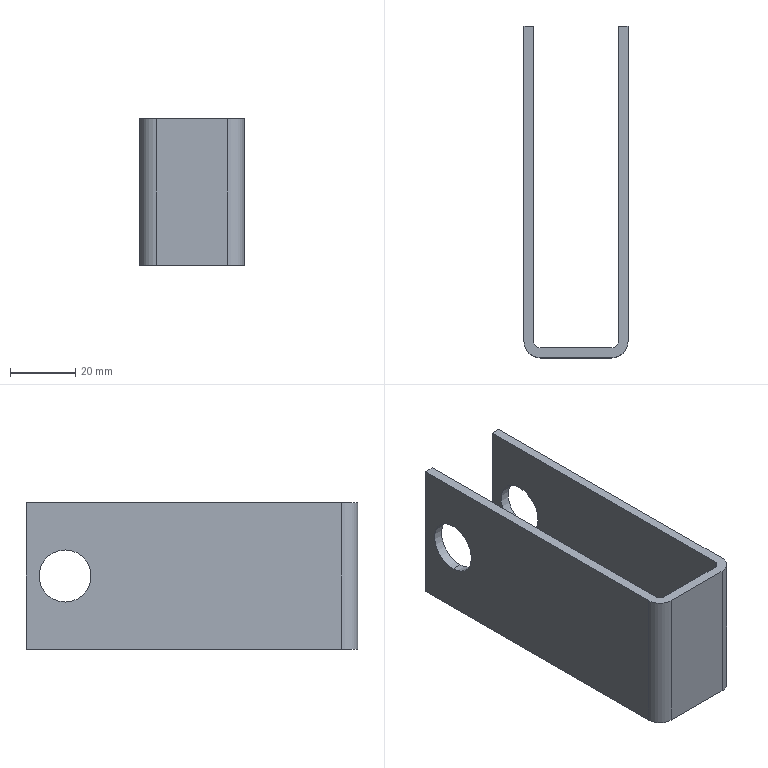Part | SolidWorks | features Extrusion 1, ICE 1 | 1 solid | 18 faces | box 32 x 102 x 45 mm | volume 29438 mm3 | plane 10 | cylinder 8 | commonest cylinder face diameters 16 x4 4 x2 10 x2
STEP:
#1=CARTESIAN_POINT('',(29.,-12.,30.5));
#2=VERTEX_POINT('',#1);
#3=CARTESIAN_POINT('',(29.,-12.,14.5));
#4=VERTEX_POINT('',#3);
#5=CARTESIAN_POINT('',(29.,-12.,22.5));
#6=DIRECTION('',(1.,0.,0.));
#7=DIRECTION('',(0.,1.,0.));
#8=AXIS2_PLACEMENT_3D('',#5,#6,#7);
#9=CIRCLE('',#8,8.);
#10=EDGE_CURVE('',#2,#4,#9,.T.);
#11=ORIENTED_EDGE('',*,*,#10,.F.);
#12=CARTESIAN_POINT('',(32.,-12.,30.5));
#13=VERTEX_POINT('',#12);
#14=CARTESIAN_POINT('',(0.,-12.,30.5));
#15=DIRECTION('',(1.,0.,0.));
#16=VECTOR('',#15,1000.);
#17=LINE('',#14,#16);
#18=EDGE_CURVE('',#2,#13,#17,.T.);
#19=ORIENTED_EDGE('',*,*,#18,.T.);
#20=CARTESIAN_POINT('',(32.,-12.,14.5));
#21=VERTEX_POINT('',#20);
#22=CARTESIAN_POINT('',(32.,-12.,22.5));
#23=DIRECTION('',(1.,0.,0.));
#24=DIRECTION('',(0.,0.,-1.));
#25=AXIS2_PLACEMENT_3D('',#22,#23,#24);
#26=CIRCLE('',#25,8.);
#27=EDGE_CURVE('',#13,#21,#26,.T.);
#28=ORIENTED_EDGE('',*,*,#27,.T.);
#29=CARTESIAN_POINT('',(0.,-12.,14.5));
#30=DIRECTION('',(1.,0.,0.));
#31=VECTOR('',#30,1000.);
#32=LINE('',#29,#31);
#33=EDGE_CURVE('',#4,#21,#32,.T.);
#34=ORIENTED_EDGE('',*,*,#33,.F.);
#35=EDGE_LOOP('',(#11,#19,#28,#34));
#36=FACE_OUTER_BOUND('',#35,.T.);
#37=CARTESIAN_POINT('',(0.,-12.,22.5));
#38=DIRECTION('',(1.,0.,0.));
#39=DIRECTION('',(0.,0.,-1.));
#40=AXIS2_PLACEMENT_3D('',#37,#38,#39);
#41=CYLINDRICAL_SURFACE('',#40,8.);
#42=ADVANCED_FACE('',(#36),#41,.F.);
#43=CARTESIAN_POINT('',(0.,-12.,30.5));
#44=VERTEX_POINT('',#43);
#45=CARTESIAN_POINT('',(0.,-12.,14.5));
#46=VERTEX_POINT('',#45);
#47=CARTESIAN_POINT('',(0.,-12.,22.5));
#48=DIRECTION('',(1.,0.,0.));
#49=DIRECTION('',(0.,0.,-1.));
#50=AXIS2_PLACEMENT_3D('',#47,#48,#49);
#51=CIRCLE('',#50,8.);
#52=EDGE_CURVE('',#44,#46,#51,.T.);
#53=ORIENTED_EDGE('',*,*,#52,.F.);
#54=CARTESIAN_POINT('',(3.,-12.,30.5));
#55=VERTEX_POINT('',#54);
#56=CARTESIAN_POINT('',(0.,-12.,30.5));
#57=DIRECTION('',(1.,0.,0.));
#58=VECTOR('',#57,1000.);
#59=LINE('',#56,#58);
#60=EDGE_CURVE('',#44,#55,#59,.T.);
#61=ORIENTED_EDGE('',*,*,#60,.T.);
#62=CARTESIAN_POINT('',(3.,-12.,14.5));
#63=VERTEX_POINT('',#62);
#64=CARTESIAN_POINT('',(3.,-12.,22.5));
#65=DIRECTION('',(-1.,0.,0.));
#66=DIRECTION('',(0.,-1.,0.));
#67=AXIS2_PLACEMENT_3D('',#64,#65,#66);
#68=CIRCLE('',#67,8.);
#69=EDGE_CURVE('',#63,#55,#68,.T.);
#70=ORIENTED_EDGE('',*,*,#69,.F.);
#71=CARTESIAN_POINT('',(0.,-12.,14.5));
#72=DIRECTION('',(1.,0.,0.));
#73=VECTOR('',#72,1000.);
#74=LINE('',#71,#73);
#75=EDGE_CURVE('',#46,#63,#74,.T.);
#76=ORIENTED_EDGE('',*,*,#75,.F.);
#77=EDGE_LOOP('',(#53,#61,#70,#76));
#78=FACE_OUTER_BOUND('',#77,.T.);
#79=CARTESIAN_POINT('',(0.,-12.,22.5));
#80=DIRECTION('',(1.,0.,0.));
#81=DIRECTION('',(0.,0.,-1.));
#82=AXIS2_PLACEMENT_3D('',#79,#80,#81);
#83=CYLINDRICAL_SURFACE('',#82,8.);
#84=ADVANCED_FACE('',(#78),#83,.F.);
#85=CARTESIAN_POINT('',(3.,0.,0.));
#86=VERTEX_POINT('',#85);
#87=CARTESIAN_POINT('',(0.,0.,0.));
#88=VERTEX_POINT('',#87);
#89=CARTESIAN_POINT('',(3.,0.,0.));
#90=DIRECTION('',(-1.,0.,0.));
#91=VECTOR('',#90,1000.);
#92=LINE('',#89,#91);
#93=EDGE_CURVE('',#86,#88,#92,.T.);
#94=ORIENTED_EDGE('',*,*,#93,.T.);
#95=CARTESIAN_POINT('',(0.,0.,45.));
#96=VERTEX_POINT('',#95);
#97=CARTESIAN_POINT('',(0.,0.,45.));
#98=DIRECTION('',(0.,0.,-1.));
#99=VECTOR('',#98,1000.);
#100=LINE('',#97,#99);
#101=EDGE_CURVE('',#96,#88,#100,.T.);
#102=ORIENTED_EDGE('',*,*,#101,.F.);
#103=CARTESIAN_POINT('',(3.,0.,45.));
#104=VERTEX_POINT('',#103);
#105=CARTESIAN_POINT('',(3.,0.,45.));
#106=DIRECTION('',(-1.,0.,0.));
#107=VECTOR('',#106,1000.);
#108=LINE('',#105,#107);
#109=EDGE_CURVE('',#104,#96,#108,.T.);
#110=ORIENTED_EDGE('',*,*,#109,.F.);
#111=CARTESIAN_POINT('',(3.,0.,45.));
#112=DIRECTION('',(0.,0.,-1.));
#113=VECTOR('',#112,1000.);
#114=LINE('',#111,#113);
#115=EDGE_CURVE('',#104,#86,#114,.T.);
#116=ORIENTED_EDGE('',*,*,#115,.T.);
#117=EDGE_LOOP('',(#94,#102,#110,#116));
#118=FACE_OUTER_BOUND('',#117,.T.);
#119=CARTESIAN_POINT('',(3.,0.,45.));
#120=DIRECTION('',(0.,-1.,0.));
#121=DIRECTION('',(0.,0.,-1.));
#122=AXIS2_PLACEMENT_3D('',#119,#120,#121);
#123=PLANE('',#122);
#124=ADVANCED_FACE('',(#118),#123,.F.);
#125=CARTESIAN_POINT('',(0.,-12.,22.5));
#126=DIRECTION('',(1.,0.,0.));
#127=DIRECTION('',(0.,0.,-1.));
#128=AXIS2_PLACEMENT_3D('',#125,#126,#127);
#129=CIRCLE('',#128,8.);
#130=EDGE_CURVE('',#46,#44,#129,.T.);
#131=ORIENTED_EDGE('',*,*,#130,.T.);
#132=ORIENTED_EDGE('',*,*,#52,.T.);
#133=EDGE_LOOP('',(#131,#132));
#134=FACE_BOUND('',#133,.T.);
#135=CARTESIAN_POINT('',(0.,-97.,0.));
#136=VERTEX_POINT('',#135);
#137=CARTESIAN_POINT('',(0.,0.,0.));
#138=DIRECTION('',(0.,-1.,0.));
#139=VECTOR('',#138,1000.);
#140=LINE('',#137,#139);
#141=EDGE_CURVE('',#88,#136,#140,.T.);
#142=ORIENTED_EDGE('',*,*,#141,.T.);
#143=CARTESIAN_POINT('',(0.,-97.,45.));
#144=VERTEX_POINT('',#143);
#145=CARTESIAN_POINT('',(0.,-97.,45.));
#146=DIRECTION('',(0.,0.,-1.));
#147=VECTOR('',#146,1000.);
#148=LINE('',#145,#147);
#149=EDGE_CURVE('',#144,#136,#148,.T.);
#150=ORIENTED_EDGE('',*,*,#149,.F.);
#151=CARTESIAN_POINT('',(0.,0.,45.));
#152=DIRECTION('',(0.,-1.,0.));
#153=VECTOR('',#152,1000.);
#154=LINE('',#151,#153);
#155=EDGE_CURVE('',#96,#144,#154,.T.);
#156=ORIENTED_EDGE('',*,*,#155,.F.);
#157=ORIENTED_EDGE('',*,*,#101,.T.);
#158=EDGE_LOOP('',(#142,#150,#156,#157));
#159=FACE_OUTER_BOUND('',#158,.T.);
#160=CARTESIAN_POINT('',(0.,0.,45.));
#161=DIRECTION('',(1.,0.,0.));
#162=DIRECTION('',(0.,1.,0.));
#163=AXIS2_PLACEMENT_3D('',#160,#161,#162);
#164=PLANE('',#163);
#165=ADVANCED_FACE('',(#134,#159),#164,.F.);
#166=CARTESIAN_POINT('',(5.,-102.,0.));
#167=VERTEX_POINT('',#166);
#168=CARTESIAN_POINT('',(5.,-97.,0.));
#169=DIRECTION('',(0.,0.,1.));
#170=DIRECTION('',(1.,0.,0.));
#171=AXIS2_PLACEMENT_3D('',#168,#169,#170);
#172=CIRCLE('',#171,5.);
#173=EDGE_CURVE('',#136,#167,#172,.T.);
#174=ORIENTED_EDGE('',*,*,#173,.T.);
#175=CARTESIAN_POINT('',(5.,-102.,45.));
#176=VERTEX_POINT('',#175);
#177=CARTESIAN_POINT('',(5.,-102.,45.));
#178=DIRECTION('',(0.,0.,-1.));
#179=VECTOR('',#178,1000.);
#180=LINE('',#177,#179);
#181=EDGE_CURVE('',#176,#167,#180,.T.);
#182=ORIENTED_EDGE('',*,*,#181,.F.);
#183=CARTESIAN_POINT('',(5.,-97.,45.));
#184=DIRECTION('',(0.,0.,1.));
#185=DIRECTION('',(1.,0.,0.));
#186=AXIS2_PLACEMENT_3D('',#183,#184,#185);
#187=CIRCLE('',#186,5.);
#188=EDGE_CURVE('',#144,#176,#187,.T.);
#189=ORIENTED_EDGE('',*,*,#188,.F.);
#190=ORIENTED_EDGE('',*,*,#149,.T.);
#191=EDGE_LOOP('',(#174,#182,#189,#190));
#192=FACE_OUTER_BOUND('',#191,.T.);
#193=CARTESIAN_POINT('',(5.,-97.,45.));
#194=DIRECTION('',(0.,0.,-1.));
#195=DIRECTION('',(-1.,0.,0.));
#196=AXIS2_PLACEMENT_3D('',#193,#194,#195);
#197=CYLINDRICAL_SURFACE('',#196,5.);
#198=ADVANCED_FACE('',(#192),#197,.T.);
#199=CARTESIAN_POINT('',(27.,-102.,0.));
#200=VERTEX_POINT('',#199);
#201=CARTESIAN_POINT('',(5.,-102.,0.));
#202=DIRECTION('',(1.,0.,0.));
#203=VECTOR('',#202,1000.);
#204=LINE('',#201,#203);
#205=EDGE_CURVE('',#167,#200,#204,.T.);
#206=ORIENTED_EDGE('',*,*,#205,.T.);
#207=CARTESIAN_POINT('',(27.,-102.,45.));
#208=VERTEX_POINT('',#207);
#209=CARTESIAN_POINT('',(27.,-102.,45.));
#210=DIRECTION('',(0.,0.,-1.));
#211=VECTOR('',#210,1000.);
#212=LINE('',#209,#211);
#213=EDGE_CURVE('',#208,#200,#212,.T.);
#214=ORIENTED_EDGE('',*,*,#213,.F.);
#215=CARTESIAN_POINT('',(5.,-102.,45.));
#216=DIRECTION('',(1.,0.,0.));
#217=VECTOR('',#216,1000.);
#218=LINE('',#215,#217);
#219=EDGE_CURVE('',#176,#208,#218,.T.);
#220=ORIENTED_EDGE('',*,*,#219,.F.);
#221=ORIENTED_EDGE('',*,*,#181,.T.);
#222=EDGE_LOOP('',(#206,#214,#220,#221));
#223=FACE_OUTER_BOUND('',#222,.T.);
#224=CARTESIAN_POINT('',(5.,-102.,45.));
#225=DIRECTION('',(0.,1.,0.));
#226=DIRECTION('',(0.,0.,1.));
#227=AXIS2_PLACEMENT_3D('',#224,#225,#226);
#228=PLANE('',#227);
#229=ADVANCED_FACE('',(#223),#228,.F.);
#230=CARTESIAN_POINT('',(32.,-97.,0.));
#231=VERTEX_POINT('',#230);
#232=CARTESIAN_POINT('',(27.,-97.,0.));
#233=DIRECTION('',(0.,0.,1.));
#234=DIRECTION('',(1.,0.,0.));
#235=AXIS2_PLACEMENT_3D('',#232,#233,#234);
#236=CIRCLE('',#235,5.);
#237=EDGE_CURVE('',#200,#231,#236,.T.);
#238=ORIENTED_EDGE('',*,*,#237,.T.);
#239=CARTESIAN_POINT('',(32.,-97.,45.));
#240=VERTEX_POINT('',#239);
#241=CARTESIAN_POINT('',(32.,-97.,45.));
#242=DIRECTION('',(0.,0.,-1.));
#243=VECTOR('',#242,1000.);
#244=LINE('',#241,#243);
#245=EDGE_CURVE('',#240,#231,#244,.T.);
#246=ORIENTED_EDGE('',*,*,#245,.F.);
#247=CARTESIAN_POINT('',(27.,-97.,45.));
#248=DIRECTION('',(0.,0.,1.));
#249=DIRECTION('',(1.,0.,0.));
#250=AXIS2_PLACEMENT_3D('',#247,#248,#249);
#251=CIRCLE('',#250,5.);
#252=EDGE_CURVE('',#208,#240,#251,.T.);
#253=ORIENTED_EDGE('',*,*,#252,.F.);
#254=ORIENTED_EDGE('',*,*,#213,.T.);
#255=EDGE_LOOP('',(#238,#246,#253,#254));
#256=FACE_OUTER_BOUND('',#255,.T.);
#257=CARTESIAN_POINT('',(27.,-97.,45.));
#258=DIRECTION('',(0.,0.,-1.));
#259=DIRECTION('',(-1.,0.,0.));
#260=AXIS2_PLACEMENT_3D('',#257,#258,#259);
#261=CYLINDRICAL_SURFACE('',#260,5.);
#262=ADVANCED_FACE('',(#256),#261,.T.);
#263=CARTESIAN_POINT('',(32.,-12.,22.5));
#264=DIRECTION('',(1.,0.,0.));
#265=DIRECTION('',(0.,0.,-1.));
#266=AXIS2_PLACEMENT_3D('',#263,#264,#265);
#267=CIRCLE('',#266,8.);
#268=EDGE_CURVE('',#21,#13,#267,.T.);
#269=ORIENTED_EDGE('',*,*,#268,.F.);
#270=ORIENTED_EDGE('',*,*,#27,.F.);
#271=EDGE_LOOP('',(#269,#270));
#272=FACE_BOUND('',#271,.T.);
#273=CARTESIAN_POINT('',(32.,0.,0.));
#274=VERTEX_POINT('',#273);
#275=CARTESIAN_POINT('',(32.,-97.,0.));
#276=DIRECTION('',(0.,1.,0.));
#277=VECTOR('',#276,1000.);
#278=LINE('',#275,#277);
#279=EDGE_CURVE('',#231,#274,#278,.T.);
#280=ORIENTED_EDGE('',*,*,#279,.T.);
#281=CARTESIAN_POINT('',(32.,0.,45.));
#282=VERTEX_POINT('',#281);
#283=CARTESIAN_POINT('',(32.,0.,45.));
#284=DIRECTION('',(0.,0.,-1.));
#285=VECTOR('',#284,1000.);
#286=LINE('',#283,#285);
#287=EDGE_CURVE('',#282,#274,#286,.T.);
#288=ORIENTED_EDGE('',*,*,#287,.F.);
#289=CARTESIAN_POINT('',(32.,-97.,45.));
#290=DIRECTION('',(0.,1.,0.));
#291=VECTOR('',#290,1000.);
#292=LINE('',#289,#291);
#293=EDGE_CURVE('',#240,#282,#292,.T.);
#294=ORIENTED_EDGE('',*,*,#293,.F.);
#295=ORIENTED_EDGE('',*,*,#245,.T.);
#296=EDGE_LOOP('',(#280,#288,#294,#295));
#297=FACE_OUTER_BOUND('',#296,.T.);
#298=CARTESIAN_POINT('',(32.,-97.,45.));
#299=DIRECTION('',(-1.,0.,0.));
#300=DIRECTION('',(0.,-1.,0.));
#301=AXIS2_PLACEMENT_3D('',#298,#299,#300);
#302=PLANE('',#301);
#303=ADVANCED_FACE('',(#272,#297),#302,.F.);
#304=CARTESIAN_POINT('',(29.,0.,0.));
#305=VERTEX_POINT('',#304);
#306=CARTESIAN_POINT('',(29.,0.,0.));
#307=DIRECTION('',(-1.,0.,0.));
#308=VECTOR('',#307,1000.);
#309=LINE('',#306,#308);
#310=EDGE_CURVE('',#274,#305,#309,.T.);
#311=ORIENTED_EDGE('',*,*,#310,.T.);
#312=CARTESIAN_POINT('',(29.,0.,45.));
#313=VERTEX_POINT('',#312);
#314=CARTESIAN_POINT('',(29.,0.,45.));
#315=DIRECTION('',(0.,0.,-1.));
#316=VECTOR('',#315,1000.);
#317=LINE('',#314,#316);
#318=EDGE_CURVE('',#313,#305,#317,.T.);
#319=ORIENTED_EDGE('',*,*,#318,.F.);
#320=CARTESIAN_POINT('',(29.,0.,45.));
#321=DIRECTION('',(-1.,0.,0.));
#322=VECTOR('',#321,1000.);
#323=LINE('',#320,#322);
#324=EDGE_CURVE('',#282,#313,#323,.T.);
#325=ORIENTED_EDGE('',*,*,#324,.F.);
#326=ORIENTED_EDGE('',*,*,#287,.T.);
#327=EDGE_LOOP('',(#311,#319,#325,#326));
#328=FACE_OUTER_BOUND('',#327,.T.);
#329=CARTESIAN_POINT('',(29.,0.,45.));
#330=DIRECTION('',(0.,-1.,0.));
#331=DIRECTION('',(1.,0.,0.));
#332=AXIS2_PLACEMENT_3D('',#329,#330,#331);
#333=PLANE('',#332);
#334=ADVANCED_FACE('',(#328),#333,.F.);
#335=CARTESIAN_POINT('',(29.,-12.,22.5));
#336=DIRECTION('',(1.,0.,0.));
#337=DIRECTION('',(0.,1.,0.));
#338=AXIS2_PLACEMENT_3D('',#335,#336,#337);
#339=CIRCLE('',#338,8.);
#340=EDGE_CURVE('',#4,#2,#339,.T.);
#341=ORIENTED_EDGE('',*,*,#340,.T.);
#342=ORIENTED_EDGE('',*,*,#10,.T.);
#343=EDGE_LOOP('',(#341,#342));
#344=FACE_BOUND('',#343,.T.);
#345=CARTESIAN_POINT('',(29.,-97.,0.));
#346=VERTEX_POINT('',#345);
#347=CARTESIAN_POINT('',(29.,-97.,0.));
#348=DIRECTION('',(0.,-1.,0.));
#349=VECTOR('',#348,1000.);
#350=LINE('',#347,#349);
#351=EDGE_CURVE('',#305,#346,#350,.T.);
#352=ORIENTED_EDGE('',*,*,#351,.T.);
#353=CARTESIAN_POINT('',(29.,-97.,45.));
#354=VERTEX_POINT('',#353);
#355=CARTESIAN_POINT('',(29.,-97.,45.));
#356=DIRECTION('',(0.,0.,-1.));
#357=VECTOR('',#356,1000.);
#358=LINE('',#355,#357);
#359=EDGE_CURVE('',#354,#346,#358,.T.);
#360=ORIENTED_EDGE('',*,*,#359,.F.);
#361=CARTESIAN_POINT('',(29.,-97.,45.));
#362=DIRECTION('',(0.,-1.,0.));
#363=VECTOR('',#362,1000.);
#364=LINE('',#361,#363);
#365=EDGE_CURVE('',#313,#354,#364,.T.);
#366=ORIENTED_EDGE('',*,*,#365,.F.);
#367=ORIENTED_EDGE('',*,*,#318,.T.);
#368=EDGE_LOOP('',(#352,#360,#366,#367));
#369=FACE_OUTER_BOUND('',#368,.T.);
#370=CARTESIAN_POINT('',(29.,-97.,45.));
#371=DIRECTION('',(1.,0.,0.));
#372=DIRECTION('',(0.,1.,0.));
#373=AXIS2_PLACEMENT_3D('',#370,#371,#372);
#374=PLANE('',#373);
#375=ADVANCED_FACE('',(#344,#369),#374,.F.);
#376=CARTESIAN_POINT('',(27.,-99.,0.));
#377=VERTEX_POINT('',#376);
#378=CARTESIAN_POINT('',(27.,-97.,0.));
#379=DIRECTION('',(0.,0.,-1.));
#380=DIRECTION('',(1.,0.,0.));
#381=AXIS2_PLACEMENT_3D('',#378,#379,#380);
#382=CIRCLE('',#381,2.);
#383=EDGE_CURVE('',#346,#377,#382,.T.);
#384=ORIENTED_EDGE('',*,*,#383,.T.);
#385=CARTESIAN_POINT('',(27.,-99.,45.));
#386=VERTEX_POINT('',#385);
#387=CARTESIAN_POINT('',(27.,-99.,45.));
#388=DIRECTION('',(0.,0.,-1.));
#389=VECTOR('',#388,1000.);
#390=LINE('',#387,#389);
#391=EDGE_CURVE('',#386,#377,#390,.T.);
#392=ORIENTED_EDGE('',*,*,#391,.F.);
#393=CARTESIAN_POINT('',(27.,-97.,45.));
#394=DIRECTION('',(0.,0.,-1.));
#395=DIRECTION('',(1.,0.,0.));
#396=AXIS2_PLACEMENT_3D('',#393,#394,#395);
#397=CIRCLE('',#396,2.);
#398=EDGE_CURVE('',#354,#386,#397,.T.);
#399=ORIENTED_EDGE('',*,*,#398,.F.);
#400=ORIENTED_EDGE('',*,*,#359,.T.);
#401=EDGE_LOOP('',(#384,#392,#399,#400));
#402=FACE_OUTER_BOUND('',#401,.T.);
#403=CARTESIAN_POINT('',(27.,-97.,45.));
#404=DIRECTION('',(0.,0.,-1.));
#405=DIRECTION('',(-1.,0.,0.));
#406=AXIS2_PLACEMENT_3D('',#403,#404,#405);
#407=CYLINDRICAL_SURFACE('',#406,2.);
#408=ADVANCED_FACE('',(#402),#407,.F.);
#409=CARTESIAN_POINT('',(5.,-99.,0.));
#410=VERTEX_POINT('',#409);
#411=CARTESIAN_POINT('',(5.,-99.,0.));
#412=DIRECTION('',(-1.,0.,0.));
#413=VECTOR('',#412,1000.);
#414=LINE('',#411,#413);
#415=EDGE_CURVE('',#377,#410,#414,.T.);
#416=ORIENTED_EDGE('',*,*,#415,.T.);
#417=CARTESIAN_POINT('',(5.,-99.,45.));
#418=VERTEX_POINT('',#417);
#419=CARTESIAN_POINT('',(5.,-99.,45.));
#420=DIRECTION('',(0.,0.,-1.));
#421=VECTOR('',#420,1000.);
#422=LINE('',#419,#421);
#423=EDGE_CURVE('',#418,#410,#422,.T.);
#424=ORIENTED_EDGE('',*,*,#423,.F.);
#425=CARTESIAN_POINT('',(5.,-99.,45.));
#426=DIRECTION('',(-1.,0.,0.));
#427=VECTOR('',#426,1000.);
#428=LINE('',#425,#427);
#429=EDGE_CURVE('',#386,#418,#428,.T.);
#430=ORIENTED_EDGE('',*,*,#429,.F.);
#431=ORIENTED_EDGE('',*,*,#391,.T.);
#432=EDGE_LOOP('',(#416,#424,#430,#431));
#433=FACE_OUTER_BOUND('',#432,.T.);
#434=CARTESIAN_POINT('',(5.,-99.,45.));
#435=DIRECTION('',(0.,-1.,0.));
#436=DIRECTION('',(0.,0.,-1.));
#437=AXIS2_PLACEMENT_3D('',#434,#435,#436);
#438=PLANE('',#437);
#439=ADVANCED_FACE('',(#433),#438,.F.);
#440=CARTESIAN_POINT('',(3.,-97.,0.));
#441=VERTEX_POINT('',#440);
#442=CARTESIAN_POINT('',(5.,-97.,0.));
#443=DIRECTION('',(0.,0.,-1.));
#444=DIRECTION('',(1.,0.,0.));
#445=AXIS2_PLACEMENT_3D('',#442,#443,#444);
#446=CIRCLE('',#445,2.);
#447=EDGE_CURVE('',#410,#441,#446,.T.);
#448=ORIENTED_EDGE('',*,*,#447,.T.);
#449=CARTESIAN_POINT('',(3.,-97.,45.));
#450=VERTEX_POINT('',#449);
#451=CARTESIAN_POINT('',(3.,-97.,45.));
#452=DIRECTION('',(0.,0.,-1.));
#453=VECTOR('',#452,1000.);
#454=LINE('',#451,#453);
#455=EDGE_CURVE('',#450,#441,#454,.T.);
#456=ORIENTED_EDGE('',*,*,#455,.F.);
#457=CARTESIAN_POINT('',(5.,-97.,45.));
#458=DIRECTION('',(0.,0.,-1.));
#459=DIRECTION('',(1.,0.,0.));
#460=AXIS2_PLACEMENT_3D('',#457,#458,#459);
#461=CIRCLE('',#460,2.);
#462=EDGE_CURVE('',#418,#450,#461,.T.);
#463=ORIENTED_EDGE('',*,*,#462,.F.);
#464=ORIENTED_EDGE('',*,*,#423,.T.);
#465=EDGE_LOOP('',(#448,#456,#463,#464));
#466=FACE_OUTER_BOUND('',#465,.T.);
#467=CARTESIAN_POINT('',(5.,-97.,45.));
#468=DIRECTION('',(0.,0.,-1.));
#469=DIRECTION('',(-1.,0.,0.));
#470=AXIS2_PLACEMENT_3D('',#467,#468,#469);
#471=CYLINDRICAL_SURFACE('',#470,2.);
#472=ADVANCED_FACE('',(#466),#471,.F.);
#473=ORIENTED_EDGE('',*,*,#69,.T.);
#474=CARTESIAN_POINT('',(3.,-12.,22.5));
#475=DIRECTION('',(-1.,0.,0.));
#476=DIRECTION('',(0.,-1.,0.));
#477=AXIS2_PLACEMENT_3D('',#474,#475,#476);
#478=CIRCLE('',#477,8.);
#479=EDGE_CURVE('',#55,#63,#478,.T.);
#480=ORIENTED_EDGE('',*,*,#479,.T.);
#481=EDGE_LOOP('',(#473,#480));
#482=FACE_BOUND('',#481,.T.);
#483=CARTESIAN_POINT('',(3.,0.,0.));
#484=DIRECTION('',(0.,1.,0.));
#485=VECTOR('',#484,1000.);
#486=LINE('',#483,#485);
#487=EDGE_CURVE('',#441,#86,#486,.T.);
#488=ORIENTED_EDGE('',*,*,#487,.T.);
#489=ORIENTED_EDGE('',*,*,#115,.F.);
#490=CARTESIAN_POINT('',(3.,0.,45.));
#491=DIRECTION('',(0.,1.,0.));
#492=VECTOR('',#491,1000.);
#493=LINE('',#490,#492);
#494=EDGE_CURVE('',#450,#104,#493,.T.);
#495=ORIENTED_EDGE('',*,*,#494,.F.);
#496=ORIENTED_EDGE('',*,*,#455,.T.);
#497=EDGE_LOOP('',(#488,#489,#495,#496));
#498=FACE_OUTER_BOUND('',#497,.T.);
#499=CARTESIAN_POINT('',(3.,0.,45.));
#500=DIRECTION('',(-1.,0.,0.));
#501=DIRECTION('',(0.,-1.,0.));
#502=AXIS2_PLACEMENT_3D('',#499,#500,#501);
#503=PLANE('',#502);
#504=ADVANCED_FACE('',(#482,#498),#503,.F.);
#505=ORIENTED_EDGE('',*,*,#109,.T.);
#506=ORIENTED_EDGE('',*,*,#155,.T.);
#507=ORIENTED_EDGE('',*,*,#188,.T.);
#508=ORIENTED_EDGE('',*,*,#219,.T.);
#509=ORIENTED_EDGE('',*,*,#252,.T.);
#510=ORIENTED_EDGE('',*,*,#293,.T.);
#511=ORIENTED_EDGE('',*,*,#324,.T.);
#512=ORIENTED_EDGE('',*,*,#365,.T.);
#513=ORIENTED_EDGE('',*,*,#398,.T.);
#514=ORIENTED_EDGE('',*,*,#429,.T.);
#515=ORIENTED_EDGE('',*,*,#462,.T.);
#516=ORIENTED_EDGE('',*,*,#494,.T.);
#517=EDGE_LOOP('',(#505,#506,#507,#508,#509,#510,#511,#512,#513,#514,#515,#516));
#518=FACE_OUTER_BOUND('',#517,.T.);
#519=CARTESIAN_POINT('',(5.,-97.,45.));
#520=DIRECTION('',(0.,0.,1.));
#521=DIRECTION('',(1.,0.,0.));
#522=AXIS2_PLACEMENT_3D('',#519,#520,#521);
#523=PLANE('',#522);
#524=ADVANCED_FACE('',(#518),#523,.T.);
#525=ORIENTED_EDGE('',*,*,#93,.F.);
#526=ORIENTED_EDGE('',*,*,#487,.F.);
#527=ORIENTED_EDGE('',*,*,#447,.F.);
#528=ORIENTED_EDGE('',*,*,#415,.F.);
#529=ORIENTED_EDGE('',*,*,#383,.F.);
#530=ORIENTED_EDGE('',*,*,#351,.F.);
#531=ORIENTED_EDGE('',*,*,#310,.F.);
#532=ORIENTED_EDGE('',*,*,#279,.F.);
#533=ORIENTED_EDGE('',*,*,#237,.F.);
#534=ORIENTED_EDGE('',*,*,#205,.F.);
#535=ORIENTED_EDGE('',*,*,#173,.F.);
#536=ORIENTED_EDGE('',*,*,#141,.F.);
#537=EDGE_LOOP('',(#525,#526,#527,#528,#529,#530,#531,#532,#533,#534,#535,#536));
#538=FACE_OUTER_BOUND('',#537,.T.);
#539=CARTESIAN_POINT('',(5.,-97.,0.));
#540=DIRECTION('',(0.,0.,1.));
#541=DIRECTION('',(1.,0.,0.));
#542=AXIS2_PLACEMENT_3D('',#539,#540,#541);
#543=PLANE('',#542);
#544=ADVANCED_FACE('',(#538),#543,.F.);
#545=ORIENTED_EDGE('',*,*,#60,.F.);
#546=ORIENTED_EDGE('',*,*,#130,.F.);
#547=ORIENTED_EDGE('',*,*,#75,.T.);
#548=ORIENTED_EDGE('',*,*,#479,.F.);
#549=EDGE_LOOP('',(#545,#546,#547,#548));
#550=FACE_OUTER_BOUND('',#549,.T.);
#551=CARTESIAN_POINT('',(0.,-12.,22.5));
#552=DIRECTION('',(1.,0.,0.));
#553=DIRECTION('',(0.,0.,-1.));
#554=AXIS2_PLACEMENT_3D('',#551,#552,#553);
#555=CYLINDRICAL_SURFACE('',#554,8.);
#556=ADVANCED_FACE('',(#550),#555,.F.);
#557=ORIENTED_EDGE('',*,*,#18,.F.);
#558=ORIENTED_EDGE('',*,*,#340,.F.);
#559=ORIENTED_EDGE('',*,*,#33,.T.);
#560=ORIENTED_EDGE('',*,*,#268,.T.);
#561=EDGE_LOOP('',(#557,#558,#559,#560));
#562=FACE_OUTER_BOUND('',#561,.T.);
#563=CARTESIAN_POINT('',(0.,-12.,22.5));
#564=DIRECTION('',(1.,0.,0.));
#565=DIRECTION('',(0.,0.,-1.));
#566=AXIS2_PLACEMENT_3D('',#563,#564,#565);
#567=CYLINDRICAL_SURFACE('',#566,8.);
#568=ADVANCED_FACE('',(#562),#567,.F.);
#569=CLOSED_SHELL('',(#42,#84,#124,#165,#198,#229,#262,#303,#334,#375,#408,#439,#472,#504,#524,#544,#556,#568));
#570=MANIFOLD_SOLID_BREP('',#569);
#571=CARTESIAN_POINT('',(0.,0.,0.));
#572=DIRECTION('',(0.,0.,1.));
#573=DIRECTION('',(1.,0.,0.));
#574=AXIS2_PLACEMENT_3D('',#571,#572,#573);
#575=(LENGTH_UNIT()NAMED_UNIT(*)SI_UNIT(.MILLI.,.METRE.));
#576=UNCERTAINTY_MEASURE_WITH_UNIT(LENGTH_MEASURE(0.00001),#575,'','');
#577=(NAMED_UNIT(*)PLANE_ANGLE_UNIT()SI_UNIT($,.RADIAN.));
#578=(NAMED_UNIT(*)SI_UNIT($,.STERADIAN.)SOLID_ANGLE_UNIT());
#579=(GEOMETRIC_REPRESENTATION_CONTEXT(3)GLOBAL_UNCERTAINTY_ASSIGNED_CONTEXT((#576))GLOBAL_UNIT_ASSIGNED_CONTEXT((#575,#577,#578))REPRESENTATION_CONTEXT('',''));
#580=ADVANCED_BREP_SHAPE_REPRESENTATION('',(#570,#574),#579);